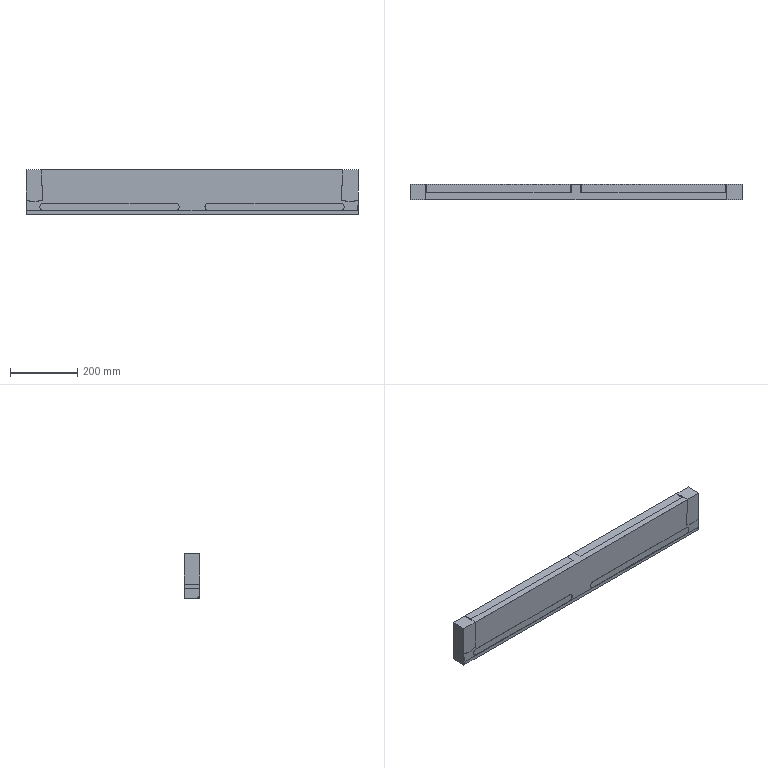NC program | NX | posted with a generic post | part box 987 x 45 x 132.5 mm
Whole program:
N10 G17 G21 G94 G90
(FLOOR_WALL , TOOL : D63)
N12 T01 M6
N14 G54
N16 G17 G0 G90 X-533. Y0. B0. C0. S6500 M3
N18 G43 Z30. H1
N20 Z3.
N22 G94 G1 Z0. F1250.
N24 X-530.
N26 X530.
N28 X533.
N30 Z3.
N32 G0 Z30.
N34 M5
(ZLEVEL_PROFILE_1_COPY_1_COPY_COPY_1 , TOOL : D10A45)
N36 T07 M6
N38 G54
N40 G17 G0 G90 X-503.04 Y25.407 B0. C0. S7500 M3
N42 G43 Z30. H7
N44 Z-0.5
N46 G94 G1 Z-1.5 F1000.
N48 X-502.37 Y24.28
N50 G3 X-501.498 Y23.79 R1.
N52 G1 X-501.283 Y23.793
N54 X501.283
N56 X501.384 Y23.782
N58 G3 X502.299 Y24.185 R1.
N60 G1 X503.149 Y25.346
N62 Z-0.5
N64 G0 Z30.
N66 X503.233 Y-25.295
N68 Z-0.5
N70 G1 Z-1.5
N72 X502.411 Y-24.173
N74 G3 X501.496 Y-23.77 R1.
N76 G1 X501.283 Y-23.793
N78 X-493.487
N80 X-501.495
N82 G3 X-502.361 Y-24.293 R1.
N84 G1 X-503.012 Y-25.42
N86 Z-0.5
N88 G0 Z30.
N90 M5
N92 M2